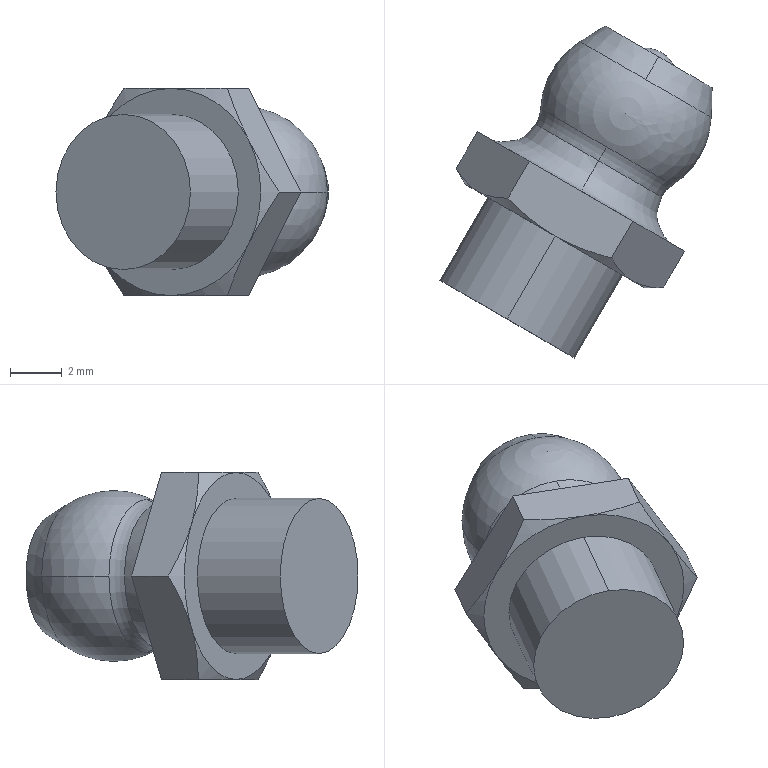Part | STEP file | uct206_021V11 | 1 solid | 28 faces | box 10.527 x 12.832 x 8 mm | volume 390.376 mm3 | plane 10 | cone 8 | torus 4 | sphere 4 | cylinder 2 | commonest cylinder face diameters 6 x2